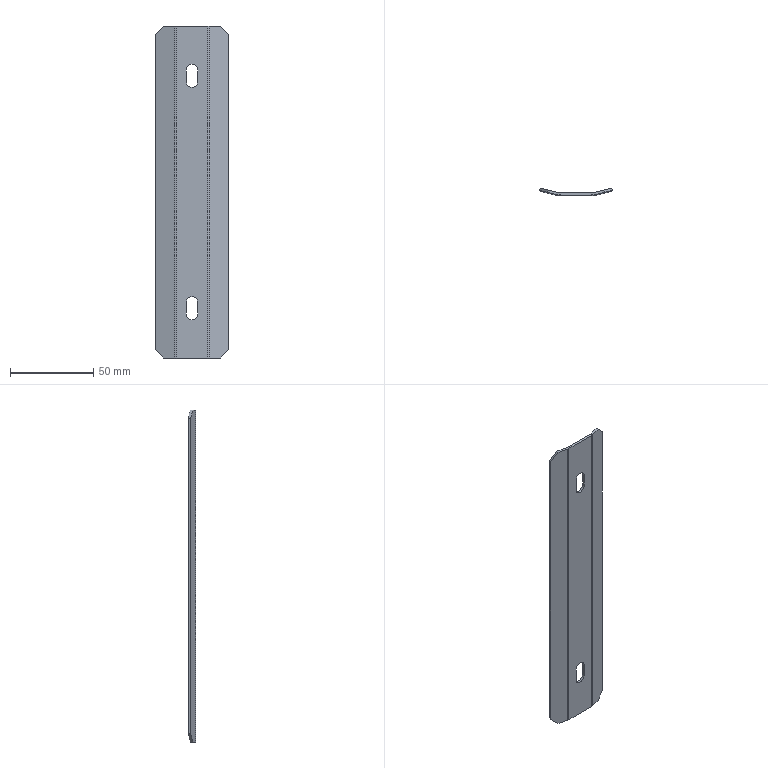Part | STEP file | SYL_0392D6J1SYL0380DJ1006_2_6-1 | 1 solid | 38 faces | box 44 x 4.447 x 200 mm | volume 12970 mm3 | plane 26 | cylinder 12 | commonest cylinder face diameters 7 x10 4 x2
STEP:
#1=CARTESIAN_POINT('',(-3.5,0.,-66.5));
#2=VERTEX_POINT('',#1);
#3=CARTESIAN_POINT('',(-3.5,1.5,-66.5));
#4=VERTEX_POINT('',#3);
#5=CARTESIAN_POINT('',(-3.5,1.5,-66.5));
#6=DIRECTION('',(0.,1.,0.));
#7=VECTOR('',#6,1000.);
#8=LINE('',#5,#7);
#9=EDGE_CURVE('',#2,#4,#8,.T.);
#10=ORIENTED_EDGE('',*,*,#9,.F.);
#11=CARTESIAN_POINT('',(-3.5,0.,-73.5));
#12=VERTEX_POINT('',#11);
#13=CARTESIAN_POINT('',(-3.5,0.,-100.));
#14=DIRECTION('',(0.,0.,-1.));
#15=VECTOR('',#14,1000.);
#16=LINE('',#13,#15);
#17=EDGE_CURVE('',#2,#12,#16,.T.);
#18=ORIENTED_EDGE('',*,*,#17,.T.);
#19=CARTESIAN_POINT('',(-3.5,1.5,-73.5));
#20=VERTEX_POINT('',#19);
#21=CARTESIAN_POINT('',(-3.5,1.5,-73.5));
#22=DIRECTION('',(0.,1.,0.));
#23=VECTOR('',#22,1000.);
#24=LINE('',#21,#23);
#25=EDGE_CURVE('',#12,#20,#24,.T.);
#26=ORIENTED_EDGE('',*,*,#25,.T.);
#27=CARTESIAN_POINT('',(-3.5,1.5,-66.5));
#28=DIRECTION('',(0.,0.,-1.));
#29=VECTOR('',#28,1000.);
#30=LINE('',#27,#29);
#31=EDGE_CURVE('',#4,#20,#30,.T.);
#32=ORIENTED_EDGE('',*,*,#31,.F.);
#33=EDGE_LOOP('',(#10,#18,#26,#32));
#34=FACE_OUTER_BOUND('',#33,.T.);
#35=CARTESIAN_POINT('',(-3.5,1.5,-66.5));
#36=DIRECTION('',(-1.,0.,0.));
#37=DIRECTION('',(0.,0.,-1.));
#38=AXIS2_PLACEMENT_3D('',#35,#36,#37);
#39=PLANE('',#38);
#40=ADVANCED_FACE('',(#34),#39,.F.);
#41=ORIENTED_EDGE('',*,*,#25,.F.);
#42=CARTESIAN_POINT('',(0.,0.,-77.));
#43=VERTEX_POINT('',#42);
#44=CARTESIAN_POINT('',(0.,0.,-73.5));
#45=DIRECTION('',(0.,-1.,0.));
#46=DIRECTION('',(0.,0.,-1.));
#47=AXIS2_PLACEMENT_3D('',#44,#45,#46);
#48=CIRCLE('',#47,3.5);
#49=EDGE_CURVE('',#12,#43,#48,.T.);
#50=ORIENTED_EDGE('',*,*,#49,.T.);
#51=CARTESIAN_POINT('',(0.,1.5,-77.));
#52=VERTEX_POINT('',#51);
#53=CARTESIAN_POINT('',(0.,1.5,-77.));
#54=DIRECTION('',(0.,1.,0.));
#55=VECTOR('',#54,1000.);
#56=LINE('',#53,#55);
#57=EDGE_CURVE('',#43,#52,#56,.T.);
#58=ORIENTED_EDGE('',*,*,#57,.T.);
#59=CARTESIAN_POINT('',(0.,1.5,-73.5));
#60=DIRECTION('',(0.,-1.,0.));
#61=DIRECTION('',(-1.,0.,0.));
#62=AXIS2_PLACEMENT_3D('',#59,#60,#61);
#63=CIRCLE('',#62,3.5);
#64=EDGE_CURVE('',#20,#52,#63,.T.);
#65=ORIENTED_EDGE('',*,*,#64,.F.);
#66=EDGE_LOOP('',(#41,#50,#58,#65));
#67=FACE_OUTER_BOUND('',#66,.T.);
#68=CARTESIAN_POINT('',(0.,1.5,-73.5));
#69=DIRECTION('',(0.,-1.,0.));
#70=DIRECTION('',(0.,0.,-1.));
#71=AXIS2_PLACEMENT_3D('',#68,#69,#70);
#72=CYLINDRICAL_SURFACE('',#71,3.5);
#73=ADVANCED_FACE('',(#67),#72,.F.);
#74=ORIENTED_EDGE('',*,*,#57,.F.);
#75=CARTESIAN_POINT('',(3.5,0.,-73.5));
#76=VERTEX_POINT('',#75);
#77=CARTESIAN_POINT('',(0.,0.,-73.5));
#78=DIRECTION('',(0.,-1.,0.));
#79=DIRECTION('',(0.,0.,-1.));
#80=AXIS2_PLACEMENT_3D('',#77,#78,#79);
#81=CIRCLE('',#80,3.5);
#82=EDGE_CURVE('',#43,#76,#81,.T.);
#83=ORIENTED_EDGE('',*,*,#82,.T.);
#84=CARTESIAN_POINT('',(3.5,1.5,-73.5));
#85=VERTEX_POINT('',#84);
#86=CARTESIAN_POINT('',(3.5,1.5,-73.5));
#87=DIRECTION('',(0.,1.,0.));
#88=VECTOR('',#87,1000.);
#89=LINE('',#86,#88);
#90=EDGE_CURVE('',#76,#85,#89,.T.);
#91=ORIENTED_EDGE('',*,*,#90,.T.);
#92=CARTESIAN_POINT('',(0.,1.5,-73.5));
#93=DIRECTION('',(0.,-1.,0.));
#94=DIRECTION('',(0.,0.,-1.));
#95=AXIS2_PLACEMENT_3D('',#92,#93,#94);
#96=CIRCLE('',#95,3.5);
#97=EDGE_CURVE('',#52,#85,#96,.T.);
#98=ORIENTED_EDGE('',*,*,#97,.F.);
#99=EDGE_LOOP('',(#74,#83,#91,#98));
#100=FACE_OUTER_BOUND('',#99,.T.);
#101=CARTESIAN_POINT('',(0.,1.5,-73.5));
#102=DIRECTION('',(0.,-1.,0.));
#103=DIRECTION('',(0.,0.,-1.));
#104=AXIS2_PLACEMENT_3D('',#101,#102,#103);
#105=CYLINDRICAL_SURFACE('',#104,3.5);
#106=ADVANCED_FACE('',(#100),#105,.F.);
#107=ORIENTED_EDGE('',*,*,#90,.F.);
#108=CARTESIAN_POINT('',(3.5,0.,-66.5));
#109=VERTEX_POINT('',#108);
#110=CARTESIAN_POINT('',(3.5,0.,-100.));
#111=DIRECTION('',(0.,0.,1.));
#112=VECTOR('',#111,1000.);
#113=LINE('',#110,#112);
#114=EDGE_CURVE('',#76,#109,#113,.T.);
#115=ORIENTED_EDGE('',*,*,#114,.T.);
#116=CARTESIAN_POINT('',(3.5,1.5,-66.5));
#117=VERTEX_POINT('',#116);
#118=CARTESIAN_POINT('',(3.5,1.5,-66.5));
#119=DIRECTION('',(0.,1.,0.));
#120=VECTOR('',#119,1000.);
#121=LINE('',#118,#120);
#122=EDGE_CURVE('',#109,#117,#121,.T.);
#123=ORIENTED_EDGE('',*,*,#122,.T.);
#124=CARTESIAN_POINT('',(3.5,1.5,-73.5));
#125=DIRECTION('',(0.,0.,1.));
#126=VECTOR('',#125,1000.);
#127=LINE('',#124,#126);
#128=EDGE_CURVE('',#85,#117,#127,.T.);
#129=ORIENTED_EDGE('',*,*,#128,.F.);
#130=EDGE_LOOP('',(#107,#115,#123,#129));
#131=FACE_OUTER_BOUND('',#130,.T.);
#132=CARTESIAN_POINT('',(3.5,1.5,-73.5));
#133=DIRECTION('',(1.,0.,0.));
#134=DIRECTION('',(0.,0.,1.));
#135=AXIS2_PLACEMENT_3D('',#132,#133,#134);
#136=PLANE('',#135);
#137=ADVANCED_FACE('',(#131),#136,.F.);
#138=ORIENTED_EDGE('',*,*,#122,.F.);
#139=CARTESIAN_POINT('',(0.,0.,-63.));
#140=VERTEX_POINT('',#139);
#141=CARTESIAN_POINT('',(0.,0.,-66.5));
#142=DIRECTION('',(0.,-1.,0.));
#143=DIRECTION('',(0.,0.,-1.));
#144=AXIS2_PLACEMENT_3D('',#141,#142,#143);
#145=CIRCLE('',#144,3.5);
#146=EDGE_CURVE('',#109,#140,#145,.T.);
#147=ORIENTED_EDGE('',*,*,#146,.T.);
#148=CARTESIAN_POINT('',(0.,1.5,-63.));
#149=VERTEX_POINT('',#148);
#150=CARTESIAN_POINT('',(0.,1.5,-63.));
#151=DIRECTION('',(0.,1.,0.));
#152=VECTOR('',#151,1000.);
#153=LINE('',#150,#152);
#154=EDGE_CURVE('',#140,#149,#153,.T.);
#155=ORIENTED_EDGE('',*,*,#154,.T.);
#156=CARTESIAN_POINT('',(0.,1.5,-66.5));
#157=DIRECTION('',(0.,-1.,0.));
#158=DIRECTION('',(1.,0.,0.));
#159=AXIS2_PLACEMENT_3D('',#156,#157,#158);
#160=CIRCLE('',#159,3.5);
#161=EDGE_CURVE('',#117,#149,#160,.T.);
#162=ORIENTED_EDGE('',*,*,#161,.F.);
#163=EDGE_LOOP('',(#138,#147,#155,#162));
#164=FACE_OUTER_BOUND('',#163,.T.);
#165=CARTESIAN_POINT('',(0.,1.5,-66.5));
#166=DIRECTION('',(0.,-1.,0.));
#167=DIRECTION('',(0.,0.,-1.));
#168=AXIS2_PLACEMENT_3D('',#165,#166,#167);
#169=CYLINDRICAL_SURFACE('',#168,3.5);
#170=ADVANCED_FACE('',(#164),#169,.F.);
#171=CARTESIAN_POINT('',(-3.5,0.,73.5));
#172=VERTEX_POINT('',#171);
#173=CARTESIAN_POINT('',(-3.5,1.5,73.5));
#174=VERTEX_POINT('',#173);
#175=CARTESIAN_POINT('',(-3.5,1.5,73.5));
#176=DIRECTION('',(0.,1.,0.));
#177=VECTOR('',#176,1000.);
#178=LINE('',#175,#177);
#179=EDGE_CURVE('',#172,#174,#178,.T.);
#180=ORIENTED_EDGE('',*,*,#179,.F.);
#181=CARTESIAN_POINT('',(-3.5,0.,66.5));
#182=VERTEX_POINT('',#181);
#183=CARTESIAN_POINT('',(-3.5,0.,-100.));
#184=DIRECTION('',(0.,0.,-1.));
#185=VECTOR('',#184,1000.);
#186=LINE('',#183,#185);
#187=EDGE_CURVE('',#172,#182,#186,.T.);
#188=ORIENTED_EDGE('',*,*,#187,.T.);
#189=CARTESIAN_POINT('',(-3.5,1.5,66.5));
#190=VERTEX_POINT('',#189);
#191=CARTESIAN_POINT('',(-3.5,1.5,66.5));
#192=DIRECTION('',(0.,1.,0.));
#193=VECTOR('',#192,1000.);
#194=LINE('',#191,#193);
#195=EDGE_CURVE('',#182,#190,#194,.T.);
#196=ORIENTED_EDGE('',*,*,#195,.T.);
#197=CARTESIAN_POINT('',(-3.5,1.5,73.5));
#198=DIRECTION('',(0.,0.,-1.));
#199=VECTOR('',#198,1000.);
#200=LINE('',#197,#199);
#201=EDGE_CURVE('',#174,#190,#200,.T.);
#202=ORIENTED_EDGE('',*,*,#201,.F.);
#203=EDGE_LOOP('',(#180,#188,#196,#202));
#204=FACE_OUTER_BOUND('',#203,.T.);
#205=CARTESIAN_POINT('',(-3.5,1.5,73.5));
#206=DIRECTION('',(-1.,0.,0.));
#207=DIRECTION('',(0.,0.,-1.));
#208=AXIS2_PLACEMENT_3D('',#205,#206,#207);
#209=PLANE('',#208);
#210=ADVANCED_FACE('',(#204),#209,.F.);
#211=ORIENTED_EDGE('',*,*,#195,.F.);
#212=CARTESIAN_POINT('',(0.,0.,63.));
#213=VERTEX_POINT('',#212);
#214=CARTESIAN_POINT('',(0.,0.,66.5));
#215=DIRECTION('',(0.,-1.,0.));
#216=DIRECTION('',(0.,0.,-1.));
#217=AXIS2_PLACEMENT_3D('',#214,#215,#216);
#218=CIRCLE('',#217,3.5);
#219=EDGE_CURVE('',#182,#213,#218,.T.);
#220=ORIENTED_EDGE('',*,*,#219,.T.);
#221=CARTESIAN_POINT('',(0.,1.5,63.));
#222=VERTEX_POINT('',#221);
#223=CARTESIAN_POINT('',(0.,1.5,63.));
#224=DIRECTION('',(0.,1.,0.));
#225=VECTOR('',#224,1000.);
#226=LINE('',#223,#225);
#227=EDGE_CURVE('',#213,#222,#226,.T.);
#228=ORIENTED_EDGE('',*,*,#227,.T.);
#229=CARTESIAN_POINT('',(0.,1.5,66.5));
#230=DIRECTION('',(0.,-1.,0.));
#231=DIRECTION('',(-1.,0.,0.));
#232=AXIS2_PLACEMENT_3D('',#229,#230,#231);
#233=CIRCLE('',#232,3.5);
#234=EDGE_CURVE('',#190,#222,#233,.T.);
#235=ORIENTED_EDGE('',*,*,#234,.F.);
#236=EDGE_LOOP('',(#211,#220,#228,#235));
#237=FACE_OUTER_BOUND('',#236,.T.);
#238=CARTESIAN_POINT('',(0.,1.5,66.5));
#239=DIRECTION('',(0.,-1.,0.));
#240=DIRECTION('',(0.,0.,-1.));
#241=AXIS2_PLACEMENT_3D('',#238,#239,#240);
#242=CYLINDRICAL_SURFACE('',#241,3.5);
#243=ADVANCED_FACE('',(#237),#242,.F.);
#244=ORIENTED_EDGE('',*,*,#227,.F.);
#245=CARTESIAN_POINT('',(3.5,0.,66.5));
#246=VERTEX_POINT('',#245);
#247=CARTESIAN_POINT('',(0.,0.,66.5));
#248=DIRECTION('',(0.,-1.,0.));
#249=DIRECTION('',(0.,0.,-1.));
#250=AXIS2_PLACEMENT_3D('',#247,#248,#249);
#251=CIRCLE('',#250,3.5);
#252=EDGE_CURVE('',#213,#246,#251,.T.);
#253=ORIENTED_EDGE('',*,*,#252,.T.);
#254=CARTESIAN_POINT('',(3.5,1.5,66.5));
#255=VERTEX_POINT('',#254);
#256=CARTESIAN_POINT('',(3.5,1.5,66.5));
#257=DIRECTION('',(0.,1.,0.));
#258=VECTOR('',#257,1000.);
#259=LINE('',#256,#258);
#260=EDGE_CURVE('',#246,#255,#259,.T.);
#261=ORIENTED_EDGE('',*,*,#260,.T.);
#262=CARTESIAN_POINT('',(0.,1.5,66.5));
#263=DIRECTION('',(0.,-1.,0.));
#264=DIRECTION('',(0.,0.,-1.));
#265=AXIS2_PLACEMENT_3D('',#262,#263,#264);
#266=CIRCLE('',#265,3.5);
#267=EDGE_CURVE('',#222,#255,#266,.T.);
#268=ORIENTED_EDGE('',*,*,#267,.F.);
#269=EDGE_LOOP('',(#244,#253,#261,#268));
#270=FACE_OUTER_BOUND('',#269,.T.);
#271=CARTESIAN_POINT('',(0.,1.5,66.5));
#272=DIRECTION('',(0.,-1.,0.));
#273=DIRECTION('',(0.,0.,-1.));
#274=AXIS2_PLACEMENT_3D('',#271,#272,#273);
#275=CYLINDRICAL_SURFACE('',#274,3.5);
#276=ADVANCED_FACE('',(#270),#275,.F.);
#277=ORIENTED_EDGE('',*,*,#260,.F.);
#278=CARTESIAN_POINT('',(3.5,0.,73.5));
#279=VERTEX_POINT('',#278);
#280=CARTESIAN_POINT('',(3.5,0.,-100.));
#281=DIRECTION('',(0.,0.,1.));
#282=VECTOR('',#281,1000.);
#283=LINE('',#280,#282);
#284=EDGE_CURVE('',#246,#279,#283,.T.);
#285=ORIENTED_EDGE('',*,*,#284,.T.);
#286=CARTESIAN_POINT('',(3.5,1.5,73.5));
#287=VERTEX_POINT('',#286);
#288=CARTESIAN_POINT('',(3.5,1.5,73.5));
#289=DIRECTION('',(0.,1.,0.));
#290=VECTOR('',#289,1000.);
#291=LINE('',#288,#290);
#292=EDGE_CURVE('',#279,#287,#291,.T.);
#293=ORIENTED_EDGE('',*,*,#292,.T.);
#294=CARTESIAN_POINT('',(3.5,1.5,66.5));
#295=DIRECTION('',(0.,0.,1.));
#296=VECTOR('',#295,1000.);
#297=LINE('',#294,#296);
#298=EDGE_CURVE('',#255,#287,#297,.T.);
#299=ORIENTED_EDGE('',*,*,#298,.F.);
#300=EDGE_LOOP('',(#277,#285,#293,#299));
#301=FACE_OUTER_BOUND('',#300,.T.);
#302=CARTESIAN_POINT('',(3.5,1.5,66.5));
#303=DIRECTION('',(1.,0.,0.));
#304=DIRECTION('',(0.,0.,1.));
#305=AXIS2_PLACEMENT_3D('',#302,#303,#304);
#306=PLANE('',#305);
#307=ADVANCED_FACE('',(#301),#306,.F.);
#308=ORIENTED_EDGE('',*,*,#292,.F.);
#309=CARTESIAN_POINT('',(0.,0.,77.));
#310=VERTEX_POINT('',#309);
#311=CARTESIAN_POINT('',(0.,0.,73.5));
#312=DIRECTION('',(0.,-1.,0.));
#313=DIRECTION('',(0.,0.,-1.));
#314=AXIS2_PLACEMENT_3D('',#311,#312,#313);
#315=CIRCLE('',#314,3.5);
#316=EDGE_CURVE('',#279,#310,#315,.T.);
#317=ORIENTED_EDGE('',*,*,#316,.T.);
#318=CARTESIAN_POINT('',(0.,1.5,77.));
#319=VERTEX_POINT('',#318);
#320=CARTESIAN_POINT('',(0.,1.5,77.));
#321=DIRECTION('',(0.,1.,0.));
#322=VECTOR('',#321,1000.);
#323=LINE('',#320,#322);
#324=EDGE_CURVE('',#310,#319,#323,.T.);
#325=ORIENTED_EDGE('',*,*,#324,.T.);
#326=CARTESIAN_POINT('',(0.,1.5,73.5));
#327=DIRECTION('',(0.,-1.,0.));
#328=DIRECTION('',(1.,0.,0.));
#329=AXIS2_PLACEMENT_3D('',#326,#327,#328);
#330=CIRCLE('',#329,3.5);
#331=EDGE_CURVE('',#287,#319,#330,.T.);
#332=ORIENTED_EDGE('',*,*,#331,.F.);
#333=EDGE_LOOP('',(#308,#317,#325,#332));
#334=FACE_OUTER_BOUND('',#333,.T.);
#335=CARTESIAN_POINT('',(0.,1.5,73.5));
#336=DIRECTION('',(0.,-1.,0.));
#337=DIRECTION('',(0.,0.,-1.));
#338=AXIS2_PLACEMENT_3D('',#335,#336,#337);
#339=CYLINDRICAL_SURFACE('',#338,3.5);
#340=ADVANCED_FACE('',(#334),#339,.F.);
#341=CARTESIAN_POINT('',(-17.149,1.782,-100.));
#342=VERTEX_POINT('',#341);
#343=CARTESIAN_POINT('',(-16.786,3.238,-100.));
#344=VERTEX_POINT('',#343);
#345=CARTESIAN_POINT('',(-16.786,3.238,-100.));
#346=DIRECTION('',(0.2419,0.9703,0.));
#347=VECTOR('',#346,1000.);
#348=LINE('',#345,#347);
#349=EDGE_CURVE('',#342,#344,#348,.T.);
#350=ORIENTED_EDGE('',*,*,#349,.F.);
#351=CARTESIAN_POINT('',(-22.,2.992,-95.));
#352=VERTEX_POINT('',#351);
#353=CARTESIAN_POINT('',(-17.149,1.782,-100.));
#354=DIRECTION('',(-0.6861,0.1711,0.7071));
#355=VECTOR('',#354,1000.);
#356=LINE('',#353,#355);
#357=EDGE_CURVE('',#342,#352,#356,.T.);
#358=ORIENTED_EDGE('',*,*,#357,.T.);
#359=CARTESIAN_POINT('',(-21.637,4.447,-95.));
#360=VERTEX_POINT('',#359);
#361=CARTESIAN_POINT('',(-21.637,4.447,-95.));
#362=DIRECTION('',(0.2419,0.9703,0.));
#363=VECTOR('',#362,1000.);
#364=LINE('',#361,#363);
#365=EDGE_CURVE('',#352,#360,#364,.T.);
#366=ORIENTED_EDGE('',*,*,#365,.T.);
#367=CARTESIAN_POINT('',(-16.786,3.238,-100.));
#368=DIRECTION('',(-0.6861,0.1711,0.7071));
#369=VECTOR('',#368,1000.);
#370=LINE('',#367,#369);
#371=EDGE_CURVE('',#344,#360,#370,.T.);
#372=ORIENTED_EDGE('',*,*,#371,.F.);
#373=EDGE_LOOP('',(#350,#358,#366,#372));
#374=FACE_OUTER_BOUND('',#373,.T.);
#375=CARTESIAN_POINT('',(-16.786,3.238,-100.));
#376=DIRECTION('',(0.6861,-0.1711,0.7071));
#377=DIRECTION('',(-0.6861,0.1711,0.7071));
#378=AXIS2_PLACEMENT_3D('',#375,#376,#377);
#379=PLANE('',#378);
#380=ADVANCED_FACE('',(#374),#379,.F.);
#381=ORIENTED_EDGE('',*,*,#365,.F.);
#382=CARTESIAN_POINT('',(-22.,2.992,95.));
#383=VERTEX_POINT('',#382);
#384=CARTESIAN_POINT('',(-22.,2.992,-100.));
#385=DIRECTION('',(0.,0.,1.));
#386=VECTOR('',#385,1000.);
#387=LINE('',#384,#386);
#388=EDGE_CURVE('',#352,#383,#387,.T.);
#389=ORIENTED_EDGE('',*,*,#388,.T.);
#390=CARTESIAN_POINT('',(-21.637,4.447,95.));
#391=VERTEX_POINT('',#390);
#392=CARTESIAN_POINT('',(-21.637,4.447,95.));
#393=DIRECTION('',(0.2419,0.9703,0.));
#394=VECTOR('',#393,1000.);
#395=LINE('',#392,#394);
#396=EDGE_CURVE('',#383,#391,#395,.T.);
#397=ORIENTED_EDGE('',*,*,#396,.T.);
#398=CARTESIAN_POINT('',(-21.637,4.447,-95.));
#399=DIRECTION('',(0.,0.,1.));
#400=VECTOR('',#399,1000.);
#401=LINE('',#398,#400);
#402=EDGE_CURVE('',#360,#391,#401,.T.);
#403=ORIENTED_EDGE('',*,*,#402,.F.);
#404=EDGE_LOOP('',(#381,#389,#397,#403));
#405=FACE_OUTER_BOUND('',#404,.T.);
#406=CARTESIAN_POINT('',(-21.637,4.447,-95.));
#407=DIRECTION('',(0.9703,-0.2419,0.));
#408=DIRECTION('',(0.,0.,1.));
#409=AXIS2_PLACEMENT_3D('',#406,#407,#408);
#410=PLANE('',#409);
#411=ADVANCED_FACE('',(#405),#410,.F.);
#412=ORIENTED_EDGE('',*,*,#396,.F.);
#413=CARTESIAN_POINT('',(-17.149,1.782,100.));
#414=VERTEX_POINT('',#413);
#415=CARTESIAN_POINT('',(-22.,2.992,95.));
#416=DIRECTION('',(0.6861,-0.1711,0.7071));
#417=VECTOR('',#416,1000.);
#418=LINE('',#415,#417);
#419=EDGE_CURVE('',#383,#414,#418,.T.);
#420=ORIENTED_EDGE('',*,*,#419,.T.);
#421=CARTESIAN_POINT('',(-16.786,3.238,100.));
#422=VERTEX_POINT('',#421);
#423=CARTESIAN_POINT('',(-16.786,3.238,100.));
#424=DIRECTION('',(0.2419,0.9703,0.));
#425=VECTOR('',#424,1000.);
#426=LINE('',#423,#425);
#427=EDGE_CURVE('',#414,#422,#426,.T.);
#428=ORIENTED_EDGE('',*,*,#427,.T.);
#429=CARTESIAN_POINT('',(-21.637,4.447,95.));
#430=DIRECTION('',(0.6861,-0.1711,0.7071));
#431=VECTOR('',#430,1000.);
#432=LINE('',#429,#431);
#433=EDGE_CURVE('',#391,#422,#432,.T.);
#434=ORIENTED_EDGE('',*,*,#433,.F.);
#435=EDGE_LOOP('',(#412,#420,#428,#434));
#436=FACE_OUTER_BOUND('',#435,.T.);
#437=CARTESIAN_POINT('',(-21.637,4.447,95.));
#438=DIRECTION('',(0.6861,-0.1711,-0.7071));
#439=DIRECTION('',(0.6861,-0.1711,0.7071));
#440=AXIS2_PLACEMENT_3D('',#437,#438,#439);
#441=PLANE('',#440);
#442=ADVANCED_FACE('',(#436),#441,.F.);
#443=ORIENTED_EDGE('',*,*,#427,.F.);
#444=CARTESIAN_POINT('',(-10.417,0.104,100.));
#445=VERTEX_POINT('',#444);
#446=CARTESIAN_POINT('',(-22.,2.992,100.));
#447=DIRECTION('',(-0.9703,0.2419,0.));
#448=VECTOR('',#447,1000.);
#449=LINE('',#446,#448);
#450=EDGE_CURVE('',#445,#414,#449,.T.);
#451=ORIENTED_EDGE('',*,*,#450,.F.);
#452=CARTESIAN_POINT('',(-10.054,1.559,100.));
#453=VERTEX_POINT('',#452);
#454=CARTESIAN_POINT('',(-10.054,1.559,100.));
#455=DIRECTION('',(0.2419,0.9703,0.));
#456=VECTOR('',#455,1000.);
#457=LINE('',#454,#456);
#458=EDGE_CURVE('',#445,#453,#457,.T.);
#459=ORIENTED_EDGE('',*,*,#458,.T.);
#460=CARTESIAN_POINT('',(-10.054,1.559,100.));
#461=DIRECTION('',(-0.9703,0.2419,0.));
#462=VECTOR('',#461,1000.);
#463=LINE('',#460,#462);
#464=EDGE_CURVE('',#453,#422,#463,.T.);
#465=ORIENTED_EDGE('',*,*,#464,.T.);
#466=EDGE_LOOP('',(#443,#451,#459,#465));
#467=FACE_OUTER_BOUND('',#466,.T.);
#468=CARTESIAN_POINT('',(-10.054,1.559,100.));
#469=DIRECTION('',(0.,0.,1.));
#470=DIRECTION('',(-0.9703,0.2419,0.));
#471=AXIS2_PLACEMENT_3D('',#468,#469,#470);
#472=PLANE('',#471);
#473=ADVANCED_FACE('',(#467),#472,.T.);
#474=ORIENTED_EDGE('',*,*,#458,.F.);
#475=CARTESIAN_POINT('',(-9.57,0.,100.));
#476=VERTEX_POINT('',#475);
#477=CARTESIAN_POINT('',(-9.57,3.5,100.));
#478=DIRECTION('',(0.,0.,-1.));
#479=DIRECTION('',(1.,0.,0.));
#480=AXIS2_PLACEMENT_3D('',#477,#478,#479);
#481=CIRCLE('',#480,3.5);
#482=EDGE_CURVE('',#476,#445,#481,.T.);
#483=ORIENTED_EDGE('',*,*,#482,.F.);
#484=CARTESIAN_POINT('',(-9.57,1.5,100.));
#485=VERTEX_POINT('',#484);
#486=CARTESIAN_POINT('',(-9.57,1.5,100.));
#487=DIRECTION('',(0.,1.,0.));
#488=VECTOR('',#487,1000.);
#489=LINE('',#486,#488);
#490=EDGE_CURVE('',#476,#485,#489,.T.);
#491=ORIENTED_EDGE('',*,*,#490,.T.);
#492=CARTESIAN_POINT('',(-9.57,3.5,100.));
#493=DIRECTION('',(0.,0.,-1.));
#494=DIRECTION('',(0.,-1.,0.));
#495=AXIS2_PLACEMENT_3D('',#492,#493,#494);
#496=CIRCLE('',#495,2.);
#497=EDGE_CURVE('',#485,#453,#496,.T.);
#498=ORIENTED_EDGE('',*,*,#497,.T.);
#499=EDGE_LOOP('',(#474,#483,#491,#498));
#500=FACE_OUTER_BOUND('',#499,.T.);
#501=CARTESIAN_POINT('',(-9.57,3.5,100.));
#502=DIRECTION('',(0.,0.,1.));
#503=DIRECTION('',(1.,0.,0.));
#504=AXIS2_PLACEMENT_3D('',#501,#502,#503);
#505=PLANE('',#504);
#506=ADVANCED_FACE('',(#500),#505,.T.);
#507=ORIENTED_EDGE('',*,*,#490,.F.);
#508=CARTESIAN_POINT('',(9.57,0.,100.));
#509=VERTEX_POINT('',#508);
#510=CARTESIAN_POINT('',(-9.57,0.,100.));
#511=DIRECTION('',(1.,0.,0.));
#512=VECTOR('',#511,1000.);
#513=LINE('',#510,#512);
#514=EDGE_CURVE('',#476,#509,#513,.T.);
#515=ORIENTED_EDGE('',*,*,#514,.T.);
#516=CARTESIAN_POINT('',(9.57,1.5,100.));
#517=VERTEX_POINT('',#516);
#518=CARTESIAN_POINT('',(9.57,0.,100.));
#519=CARTESIAN_POINT('',(9.57,0.5,100.));
#520=CARTESIAN_POINT('',(9.57,1.,100.));
#521=CARTESIAN_POINT('',(9.57,1.5,100.));
#522=B_SPLINE_CURVE_WITH_KNOTS('',3,(#518,#519,#520,#521),.UNSPECIFIED.,.F.,.F.,(4,4),(0.,1.),.UNSPECIFIED.);
#523=EDGE_CURVE('',#509,#517,#522,.T.);
#524=ORIENTED_EDGE('',*,*,#523,.T.);
#525=CARTESIAN_POINT('',(-9.57,1.5,100.));
#526=DIRECTION('',(1.,0.,0.));
#527=VECTOR('',#526,1000.);
#528=LINE('',#525,#527);
#529=EDGE_CURVE('',#485,#517,#528,.T.);
#530=ORIENTED_EDGE('',*,*,#529,.F.);
#531=EDGE_LOOP('',(#507,#515,#524,#530));
#532=FACE_OUTER_BOUND('',#531,.T.);
#533=CARTESIAN_POINT('',(-9.57,1.5,100.));
#534=DIRECTION('',(0.,0.,-1.));
#535=DIRECTION('',(1.,0.,0.));
#536=AXIS2_PLACEMENT_3D('',#533,#534,#535);
#537=PLANE('',#536);
#538=ADVANCED_FACE('',(#532),#537,.F.);
#539=ORIENTED_EDGE('',*,*,#523,.F.);
#540=CARTESIAN_POINT('',(10.421,0.1051,100.));
#541=VERTEX_POINT('',#540);
#542=CARTESIAN_POINT('',(10.421,0.1051,100.));
#543=CARTESIAN_POINT('',(10.143,0.03537,100.));
#544=CARTESIAN_POINT('',(9.857,0.,100.));
#545=CARTESIAN_POINT('',(9.57,0.,100.));
#546=B_SPLINE_CURVE_WITH_KNOTS('',3,(#542,#543,#544,#545),.UNSPECIFIED.,.F.,.F.,(4,4),(0.,1.),.UNSPECIFIED.);
#547=EDGE_CURVE('',#541,#509,#546,.T.);
#548=ORIENTED_EDGE('',*,*,#547,.F.);
#549=CARTESIAN_POINT('',(10.057,1.56,100.));
#550=VERTEX_POINT('',#549);
#551=CARTESIAN_POINT('',(10.421,0.1051,100.));
#552=CARTESIAN_POINT('',(10.3,0.59,100.));
#553=CARTESIAN_POINT('',(10.178,1.075,100.));
#554=CARTESIAN_POINT('',(10.057,1.56,100.));
#555=B_SPLINE_CURVE_WITH_KNOTS('',3,(#551,#552,#553,#554),.UNSPECIFIED.,.F.,.F.,(4,4),(0.,1.),.UNSPECIFIED.);
#556=EDGE_CURVE('',#541,#550,#555,.T.);
#557=ORIENTED_EDGE('',*,*,#556,.T.);
#558=CARTESIAN_POINT('',(10.057,1.56,100.));
#559=CARTESIAN_POINT('',(9.897,1.52,100.));
#560=CARTESIAN_POINT('',(9.735,1.5,100.));
#561=CARTESIAN_POINT('',(9.57,1.5,100.));
#562=B_SPLINE_CURVE_WITH_KNOTS('',3,(#558,#559,#560,#561),.UNSPECIFIED.,.F.,.F.,(4,4),(0.,1.),.UNSPECIFIED.);
#563=EDGE_CURVE('',#550,#517,#562,.T.);
#564=ORIENTED_EDGE('',*,*,#563,.T.);
#565=EDGE_LOOP('',(#539,#548,#557,#564));
#566=FACE_OUTER_BOUND('',#565,.T.);
#567=CARTESIAN_POINT('',(9.57,3.5,100.));
#568=DIRECTION('',(0.,0.,-1.));
#569=DIRECTION('',(-1.,0.,0.));
#570=AXIS2_PLACEMENT_3D('',#567,#568,#569);
#571=PLANE('',#570);
#572=ADVANCED_FACE('',(#566),#571,.F.);
#573=ORIENTED_EDGE('',*,*,#556,.F.);
#574=CARTESIAN_POINT('',(17.149,1.782,100.));
#575=VERTEX_POINT('',#574);
#576=CARTESIAN_POINT('',(10.417,0.104,100.));
#577=DIRECTION('',(-0.9703,-0.2419,0.));
#578=VECTOR('',#577,1000.);
#579=LINE('',#576,#578);
#580=EDGE_CURVE('',#575,#541,#579,.T.);
#581=ORIENTED_EDGE('',*,*,#580,.F.);
#582=CARTESIAN_POINT('',(16.786,3.238,100.));
#583=VERTEX_POINT('',#582);
#584=CARTESIAN_POINT('',(16.786,3.238,100.));
#585=DIRECTION('',(-0.2419,0.9703,0.));
#586=VECTOR('',#585,1000.);
#587=LINE('',#584,#586);
#588=EDGE_CURVE('',#575,#583,#587,.T.);
#589=ORIENTED_EDGE('',*,*,#588,.T.);
#590=CARTESIAN_POINT('',(16.786,3.238,100.));
#591=DIRECTION('',(-0.9703,-0.2419,0.));
#592=VECTOR('',#591,1000.);
#593=LINE('',#590,#592);
#594=EDGE_CURVE('',#583,#550,#593,.T.);
#595=ORIENTED_EDGE('',*,*,#594,.T.);
#596=EDGE_LOOP('',(#573,#581,#589,#595));
#597=FACE_OUTER_BOUND('',#596,.T.);
#598=CARTESIAN_POINT('',(16.786,3.238,100.));
#599=DIRECTION('',(0.,0.,1.));
#600=DIRECTION('',(-0.9703,-0.2419,0.));
#601=AXIS2_PLACEMENT_3D('',#598,#599,#600);
#602=PLANE('',#601);
#603=ADVANCED_FACE('',(#597),#602,.T.);
#604=ORIENTED_EDGE('',*,*,#588,.F.);
#605=CARTESIAN_POINT('',(22.,2.992,95.));
#606=VERTEX_POINT('',#605);
#607=CARTESIAN_POINT('',(17.149,1.782,100.));
#608=DIRECTION('',(0.6861,0.1711,-0.7071));
#609=VECTOR('',#608,1000.);
#610=LINE('',#607,#609);
#611=EDGE_CURVE('',#575,#606,#610,.T.);
#612=ORIENTED_EDGE('',*,*,#611,.T.);
#613=CARTESIAN_POINT('',(21.637,4.447,95.));
#614=VERTEX_POINT('',#613);
#615=CARTESIAN_POINT('',(21.637,4.447,95.));
#616=DIRECTION('',(-0.2419,0.9703,0.));
#617=VECTOR('',#616,1000.);
#618=LINE('',#615,#617);
#619=EDGE_CURVE('',#606,#614,#618,.T.);
#620=ORIENTED_EDGE('',*,*,#619,.T.);
#621=CARTESIAN_POINT('',(16.786,3.238,100.));
#622=DIRECTION('',(0.6861,0.1711,-0.7071));
#623=VECTOR('',#622,1000.);
#624=LINE('',#621,#623);
#625=EDGE_CURVE('',#583,#614,#624,.T.);
#626=ORIENTED_EDGE('',*,*,#625,.F.);
#627=EDGE_LOOP('',(#604,#612,#620,#626));
#628=FACE_OUTER_BOUND('',#627,.T.);
#629=CARTESIAN_POINT('',(16.786,3.238,100.));
#630=DIRECTION('',(-0.6861,-0.1711,-0.7071));
#631=DIRECTION('',(0.6861,0.1711,-0.7071));
#632=AXIS2_PLACEMENT_3D('',#629,#630,#631);
#633=PLANE('',#632);
#634=ADVANCED_FACE('',(#628),#633,.F.);
#635=ORIENTED_EDGE('',*,*,#619,.F.);
#636=CARTESIAN_POINT('',(22.,2.992,-95.));
#637=VERTEX_POINT('',#636);
#638=CARTESIAN_POINT('',(22.,2.992,-100.));
#639=DIRECTION('',(0.,0.,-1.));
#640=VECTOR('',#639,1000.);
#641=LINE('',#638,#640);
#642=EDGE_CURVE('',#606,#637,#641,.T.);
#643=ORIENTED_EDGE('',*,*,#642,.T.);
#644=CARTESIAN_POINT('',(21.637,4.447,-95.));
#645=VERTEX_POINT('',#644);
#646=CARTESIAN_POINT('',(21.637,4.447,-95.));
#647=DIRECTION('',(-0.2419,0.9703,0.));
#648=VECTOR('',#647,1000.);
#649=LINE('',#646,#648);
#650=EDGE_CURVE('',#637,#645,#649,.T.);
#651=ORIENTED_EDGE('',*,*,#650,.T.);
#652=CARTESIAN_POINT('',(21.637,4.447,95.));
#653=DIRECTION('',(0.,0.,-1.));
#654=VECTOR('',#653,1000.);
#655=LINE('',#652,#654);
#656=EDGE_CURVE('',#614,#645,#655,.T.);
#657=ORIENTED_EDGE('',*,*,#656,.F.);
#658=EDGE_LOOP('',(#635,#643,#651,#657));
#659=FACE_OUTER_BOUND('',#658,.T.);
#660=CARTESIAN_POINT('',(21.637,4.447,95.));
#661=DIRECTION('',(-0.9703,-0.2419,0.));
#662=DIRECTION('',(0.,0.,-1.));
#663=AXIS2_PLACEMENT_3D('',#660,#661,#662);
#664=PLANE('',#663);
#665=ADVANCED_FACE('',(#659),#664,.F.);
#666=ORIENTED_EDGE('',*,*,#650,.F.);
#667=CARTESIAN_POINT('',(17.149,1.782,-100.));
#668=VERTEX_POINT('',#667);
#669=CARTESIAN_POINT('',(22.,2.992,-95.));
#670=DIRECTION('',(-0.6861,-0.1711,-0.7071));
#671=VECTOR('',#670,1000.);
#672=LINE('',#669,#671);
#673=EDGE_CURVE('',#637,#668,#672,.T.);
#674=ORIENTED_EDGE('',*,*,#673,.T.);
#675=CARTESIAN_POINT('',(16.786,3.238,-100.));
#676=VERTEX_POINT('',#675);
#677=CARTESIAN_POINT('',(16.786,3.238,-100.));
#678=DIRECTION('',(-0.2419,0.9703,0.));
#679=VECTOR('',#678,1000.);
#680=LINE('',#677,#679);
#681=EDGE_CURVE('',#668,#676,#680,.T.);
#682=ORIENTED_EDGE('',*,*,#681,.T.);
#683=CARTESIAN_POINT('',(21.637,4.447,-95.));
#684=DIRECTION('',(-0.6861,-0.1711,-0.7071));
#685=VECTOR('',#684,1000.);
#686=LINE('',#683,#685);
#687=EDGE_CURVE('',#645,#676,#686,.T.);
#688=ORIENTED_EDGE('',*,*,#687,.F.);
#689=EDGE_LOOP('',(#666,#674,#682,#688));
#690=FACE_OUTER_BOUND('',#689,.T.);
#691=CARTESIAN_POINT('',(21.637,4.447,-95.));
#692=DIRECTION('',(-0.6861,-0.1711,0.7071));
#693=DIRECTION('',(-0.6861,-0.1711,-0.7071));
#694=AXIS2_PLACEMENT_3D('',#691,#692,#693);
#695=PLANE('',#694);
#696=ADVANCED_FACE('',(#690),#695,.F.);
#697=ORIENTED_EDGE('',*,*,#681,.F.);
#698=CARTESIAN_POINT('',(10.421,0.1051,-100.));
#699=VERTEX_POINT('',#698);
#700=CARTESIAN_POINT('',(10.417,0.104,-100.));
#701=DIRECTION('',(0.9703,0.2419,0.));
#702=VECTOR('',#701,1000.);
#703=LINE('',#700,#702);
#704=EDGE_CURVE('',#699,#668,#703,.T.);
#705=ORIENTED_EDGE('',*,*,#704,.F.);
#706=CARTESIAN_POINT('',(10.057,1.56,-100.));
#707=VERTEX_POINT('',#706);
#708=CARTESIAN_POINT('',(10.421,0.1051,-100.));
#709=CARTESIAN_POINT('',(10.3,0.59,-100.));
#710=CARTESIAN_POINT('',(10.178,1.075,-100.));
#711=CARTESIAN_POINT('',(10.057,1.56,-100.));
#712=B_SPLINE_CURVE_WITH_KNOTS('',3,(#708,#709,#710,#711),.UNSPECIFIED.,.F.,.F.,(4,4),(0.,1.),.UNSPECIFIED.);
#713=EDGE_CURVE('',#699,#707,#712,.T.);
#714=ORIENTED_EDGE('',*,*,#713,.T.);
#715=CARTESIAN_POINT('',(10.057,1.56,-100.));
#716=DIRECTION('',(0.9703,0.2419,0.));
#717=VECTOR('',#716,1000.);
#718=LINE('',#715,#717);
#719=EDGE_CURVE('',#707,#676,#718,.T.);
#720=ORIENTED_EDGE('',*,*,#719,.T.);
#721=EDGE_LOOP('',(#697,#705,#714,#720));
#722=FACE_OUTER_BOUND('',#721,.T.);
#723=CARTESIAN_POINT('',(10.057,1.56,-100.));
#724=DIRECTION('',(0.,0.,-1.));
#725=DIRECTION('',(0.9703,0.2419,0.));
#726=AXIS2_PLACEMENT_3D('',#723,#724,#725);
#727=PLANE('',#726);
#728=ADVANCED_FACE('',(#722),#727,.T.);
#729=ORIENTED_EDGE('',*,*,#713,.F.);
#730=CARTESIAN_POINT('',(9.57,0.,-100.));
#731=VERTEX_POINT('',#730);
#732=CARTESIAN_POINT('',(9.57,0.,-100.));
#733=CARTESIAN_POINT('',(9.857,0.,-100.));
#734=CARTESIAN_POINT('',(10.143,0.03537,-100.));
#735=CARTESIAN_POINT('',(10.421,0.1051,-100.));
#736=B_SPLINE_CURVE_WITH_KNOTS('',3,(#732,#733,#734,#735),.UNSPECIFIED.,.F.,.F.,(4,4),(0.,1.),.UNSPECIFIED.);
#737=EDGE_CURVE('',#731,#699,#736,.T.);
#738=ORIENTED_EDGE('',*,*,#737,.F.);
#739=CARTESIAN_POINT('',(9.57,1.5,-100.));
#740=VERTEX_POINT('',#739);
#741=CARTESIAN_POINT('',(9.57,0.,-100.));
#742=CARTESIAN_POINT('',(9.57,0.5,-100.));
#743=CARTESIAN_POINT('',(9.57,1.,-100.));
#744=CARTESIAN_POINT('',(9.57,1.5,-100.));
#745=B_SPLINE_CURVE_WITH_KNOTS('',3,(#741,#742,#743,#744),.UNSPECIFIED.,.F.,.F.,(4,4),(0.,1.),.UNSPECIFIED.);
#746=EDGE_CURVE('',#731,#740,#745,.T.);
#747=ORIENTED_EDGE('',*,*,#746,.T.);
#748=CARTESIAN_POINT('',(9.57,1.5,-100.));
#749=CARTESIAN_POINT('',(9.735,1.5,-100.));
#750=CARTESIAN_POINT('',(9.897,1.52,-100.));
#751=CARTESIAN_POINT('',(10.057,1.56,-100.));
#752=B_SPLINE_CURVE_WITH_KNOTS('',3,(#748,#749,#750,#751),.UNSPECIFIED.,.F.,.F.,(4,4),(0.,1.),.UNSPECIFIED.);
#753=EDGE_CURVE('',#740,#707,#752,.T.);
#754=ORIENTED_EDGE('',*,*,#753,.T.);
#755=EDGE_LOOP('',(#729,#738,#747,#754));
#756=FACE_OUTER_BOUND('',#755,.T.);
#757=CARTESIAN_POINT('',(9.57,3.5,-100.));
#758=DIRECTION('',(0.,0.,-1.));
#759=DIRECTION('',(-1.,0.,0.));
#760=AXIS2_PLACEMENT_3D('',#757,#758,#759);
#761=PLANE('',#760);
#762=ADVANCED_FACE('',(#756),#761,.T.);
#763=ORIENTED_EDGE('',*,*,#746,.F.);
#764=CARTESIAN_POINT('',(-9.57,0.,-100.));
#765=VERTEX_POINT('',#764);
#766=CARTESIAN_POINT('',(-9.57,0.,-100.));
#767=DIRECTION('',(-1.,0.,0.));
#768=VECTOR('',#767,1000.);
#769=LINE('',#766,#768);
#770=EDGE_CURVE('',#731,#765,#769,.T.);
#771=ORIENTED_EDGE('',*,*,#770,.T.);
#772=CARTESIAN_POINT('',(-9.57,1.5,-100.));
#773=VERTEX_POINT('',#772);
#774=CARTESIAN_POINT('',(-9.57,1.5,-100.));
#775=DIRECTION('',(0.,1.,0.));
#776=VECTOR('',#775,1000.);
#777=LINE('',#774,#776);
#778=EDGE_CURVE('',#765,#773,#777,.T.);
#779=ORIENTED_EDGE('',*,*,#778,.T.);
#780=CARTESIAN_POINT('',(9.57,1.5,-100.));
#781=DIRECTION('',(-1.,0.,0.));
#782=VECTOR('',#781,1000.);
#783=LINE('',#780,#782);
#784=EDGE_CURVE('',#740,#773,#783,.T.);
#785=ORIENTED_EDGE('',*,*,#784,.F.);
#786=EDGE_LOOP('',(#763,#771,#779,#785));
#787=FACE_OUTER_BOUND('',#786,.T.);
#788=CARTESIAN_POINT('',(9.57,1.5,-100.));
#789=DIRECTION('',(0.,0.,1.));
#790=DIRECTION('',(-1.,0.,0.));
#791=AXIS2_PLACEMENT_3D('',#788,#789,#790);
#792=PLANE('',#791);
#793=ADVANCED_FACE('',(#787),#792,.F.);
#794=ORIENTED_EDGE('',*,*,#778,.F.);
#795=CARTESIAN_POINT('',(-10.417,0.104,-100.));
#796=VERTEX_POINT('',#795);
#797=CARTESIAN_POINT('',(-9.57,3.5,-100.));
#798=DIRECTION('',(0.,0.,1.));
#799=DIRECTION('',(1.,0.,0.));
#800=AXIS2_PLACEMENT_3D('',#797,#798,#799);
#801=CIRCLE('',#800,3.5);
#802=EDGE_CURVE('',#796,#765,#801,.T.);
#803=ORIENTED_EDGE('',*,*,#802,.F.);
#804=CARTESIAN_POINT('',(-10.054,1.559,-100.));
#805=VERTEX_POINT('',#804);
#806=CARTESIAN_POINT('',(-10.054,1.559,-100.));
#807=DIRECTION('',(0.2419,0.9703,0.));
#808=VECTOR('',#807,1000.);
#809=LINE('',#806,#808);
#810=EDGE_CURVE('',#796,#805,#809,.T.);
#811=ORIENTED_EDGE('',*,*,#810,.T.);
#812=CARTESIAN_POINT('',(-9.57,3.5,-100.));
#813=DIRECTION('',(0.,0.,1.));
#814=DIRECTION('',(-0.2419,-0.9703,0.));
#815=AXIS2_PLACEMENT_3D('',#812,#813,#814);
#816=CIRCLE('',#815,2.);
#817=EDGE_CURVE('',#805,#773,#816,.T.);
#818=ORIENTED_EDGE('',*,*,#817,.T.);
#819=EDGE_LOOP('',(#794,#803,#811,#818));
#820=FACE_OUTER_BOUND('',#819,.T.);
#821=CARTESIAN_POINT('',(-9.57,3.5,-100.));
#822=DIRECTION('',(0.,0.,-1.));
#823=DIRECTION('',(-1.,0.,0.));
#824=AXIS2_PLACEMENT_3D('',#821,#822,#823);
#825=PLANE('',#824);
#826=ADVANCED_FACE('',(#820),#825,.T.);
#827=CARTESIAN_POINT('',(0.,0.,73.5));
#828=DIRECTION('',(0.,-1.,0.));
#829=DIRECTION('',(0.,0.,-1.));
#830=AXIS2_PLACEMENT_3D('',#827,#828,#829);
#831=CIRCLE('',#830,3.5);
#832=EDGE_CURVE('',#310,#172,#831,.T.);
#833=ORIENTED_EDGE('',*,*,#832,.T.);
#834=ORIENTED_EDGE('',*,*,#179,.T.);
#835=CARTESIAN_POINT('',(0.,1.5,73.5));
#836=DIRECTION('',(0.,-1.,0.));
#837=DIRECTION('',(0.,0.,1.));
#838=AXIS2_PLACEMENT_3D('',#835,#836,#837);
#839=CIRCLE('',#838,3.5);
#840=EDGE_CURVE('',#319,#174,#839,.T.);
#841=ORIENTED_EDGE('',*,*,#840,.F.);
#842=ORIENTED_EDGE('',*,*,#324,.F.);
#843=EDGE_LOOP('',(#833,#834,#841,#842));
#844=FACE_OUTER_BOUND('',#843,.T.);
#845=CARTESIAN_POINT('',(0.,1.5,73.5));
#846=DIRECTION('',(0.,-1.,0.));
#847=DIRECTION('',(0.,0.,-1.));
#848=AXIS2_PLACEMENT_3D('',#845,#846,#847);
#849=CYLINDRICAL_SURFACE('',#848,3.5);
#850=ADVANCED_FACE('',(#844),#849,.F.);
#851=CARTESIAN_POINT('',(0.,0.,-66.5));
#852=DIRECTION('',(0.,-1.,0.));
#853=DIRECTION('',(0.,0.,-1.));
#854=AXIS2_PLACEMENT_3D('',#851,#852,#853);
#855=CIRCLE('',#854,3.5);
#856=EDGE_CURVE('',#140,#2,#855,.T.);
#857=ORIENTED_EDGE('',*,*,#856,.T.);
#858=ORIENTED_EDGE('',*,*,#9,.T.);
#859=CARTESIAN_POINT('',(0.,1.5,-66.5));
#860=DIRECTION('',(0.,-1.,0.));
#861=DIRECTION('',(0.,0.,1.));
#862=AXIS2_PLACEMENT_3D('',#859,#860,#861);
#863=CIRCLE('',#862,3.5);
#864=EDGE_CURVE('',#149,#4,#863,.T.);
#865=ORIENTED_EDGE('',*,*,#864,.F.);
#866=ORIENTED_EDGE('',*,*,#154,.F.);
#867=EDGE_LOOP('',(#857,#858,#865,#866));
#868=FACE_OUTER_BOUND('',#867,.T.);
#869=CARTESIAN_POINT('',(0.,1.5,-66.5));
#870=DIRECTION('',(0.,-1.,0.));
#871=DIRECTION('',(0.,0.,-1.));
#872=AXIS2_PLACEMENT_3D('',#869,#870,#871);
#873=CYLINDRICAL_SURFACE('',#872,3.5);
#874=ADVANCED_FACE('',(#868),#873,.F.);
#875=CARTESIAN_POINT('',(-22.,2.992,-100.));
#876=DIRECTION('',(0.9703,-0.2419,0.));
#877=VECTOR('',#876,1000.);
#878=LINE('',#875,#877);
#879=EDGE_CURVE('',#342,#796,#878,.T.);
#880=ORIENTED_EDGE('',*,*,#879,.F.);
#881=ORIENTED_EDGE('',*,*,#349,.T.);
#882=CARTESIAN_POINT('',(-16.786,3.238,-100.));
#883=DIRECTION('',(0.9703,-0.2419,0.));
#884=VECTOR('',#883,1000.);
#885=LINE('',#882,#884);
#886=EDGE_CURVE('',#344,#805,#885,.T.);
#887=ORIENTED_EDGE('',*,*,#886,.T.);
#888=ORIENTED_EDGE('',*,*,#810,.F.);
#889=EDGE_LOOP('',(#880,#881,#887,#888));
#890=FACE_OUTER_BOUND('',#889,.T.);
#891=CARTESIAN_POINT('',(-16.786,3.238,-100.));
#892=DIRECTION('',(0.,0.,-1.));
#893=DIRECTION('',(0.9703,-0.2419,0.));
#894=AXIS2_PLACEMENT_3D('',#891,#892,#893);
#895=PLANE('',#894);
#896=ADVANCED_FACE('',(#890),#895,.T.);
#897=CARTESIAN_POINT('',(-9.57,1.5,100.));
#898=DIRECTION('',(0.,0.,-1.));
#899=VECTOR('',#898,1000.);
#900=LINE('',#897,#899);
#901=EDGE_CURVE('',#485,#773,#900,.T.);
#902=ORIENTED_EDGE('',*,*,#901,.T.);
#903=ORIENTED_EDGE('',*,*,#817,.F.);
#904=CARTESIAN_POINT('',(-10.054,1.559,-100.));
#905=DIRECTION('',(0.,0.,1.));
#906=VECTOR('',#905,1000.);
#907=LINE('',#904,#906);
#908=EDGE_CURVE('',#805,#453,#907,.T.);
#909=ORIENTED_EDGE('',*,*,#908,.T.);
#910=ORIENTED_EDGE('',*,*,#497,.F.);
#911=EDGE_LOOP('',(#902,#903,#909,#910));
#912=FACE_OUTER_BOUND('',#911,.T.);
#913=CARTESIAN_POINT('',(-9.57,3.5,-100.));
#914=DIRECTION('',(0.,0.,1.));
#915=DIRECTION('',(1.,0.,0.));
#916=AXIS2_PLACEMENT_3D('',#913,#914,#915);
#917=CYLINDRICAL_SURFACE('',#916,2.);
#918=ADVANCED_FACE('',(#912),#917,.F.);
#919=ORIENTED_EDGE('',*,*,#464,.F.);
#920=ORIENTED_EDGE('',*,*,#908,.F.);
#921=ORIENTED_EDGE('',*,*,#886,.F.);
#922=ORIENTED_EDGE('',*,*,#371,.T.);
#923=ORIENTED_EDGE('',*,*,#402,.T.);
#924=ORIENTED_EDGE('',*,*,#433,.T.);
#925=EDGE_LOOP('',(#919,#920,#921,#922,#923,#924));
#926=FACE_OUTER_BOUND('',#925,.T.);
#927=CARTESIAN_POINT('',(-21.637,4.447,-100.));
#928=DIRECTION('',(-0.2419,-0.9703,0.));
#929=DIRECTION('',(-0.9703,0.2419,0.));
#930=AXIS2_PLACEMENT_3D('',#927,#928,#929);
#931=PLANE('',#930);
#932=ADVANCED_FACE('',(#926),#931,.F.);
#933=CARTESIAN_POINT('',(10.057,1.56,100.));
#934=DIRECTION('',(0.,0.,-1.));
#935=VECTOR('',#934,1000.);
#936=LINE('',#933,#935);
#937=EDGE_CURVE('',#550,#707,#936,.T.);
#938=ORIENTED_EDGE('',*,*,#937,.T.);
#939=ORIENTED_EDGE('',*,*,#753,.F.);
#940=CARTESIAN_POINT('',(9.57,1.5,-100.));
#941=DIRECTION('',(0.,0.,1.));
#942=VECTOR('',#941,1000.);
#943=LINE('',#940,#942);
#944=EDGE_CURVE('',#740,#517,#943,.T.);
#945=ORIENTED_EDGE('',*,*,#944,.T.);
#946=ORIENTED_EDGE('',*,*,#563,.F.);
#947=EDGE_LOOP('',(#938,#939,#945,#946));
#948=FACE_OUTER_BOUND('',#947,.T.);
#949=CARTESIAN_POINT('',(9.57,3.5,-100.));
#950=DIRECTION('',(0.,0.,1.));
#951=DIRECTION('',(1.,0.,0.));
#952=AXIS2_PLACEMENT_3D('',#949,#950,#951);
#953=CYLINDRICAL_SURFACE('',#952,2.);
#954=ADVANCED_FACE('',(#948),#953,.F.);
#955=ORIENTED_EDGE('',*,*,#331,.T.);
#956=ORIENTED_EDGE('',*,*,#840,.T.);
#957=ORIENTED_EDGE('',*,*,#201,.T.);
#958=ORIENTED_EDGE('',*,*,#234,.T.);
#959=ORIENTED_EDGE('',*,*,#267,.T.);
#960=ORIENTED_EDGE('',*,*,#298,.T.);
#961=EDGE_LOOP('',(#955,#956,#957,#958,#959,#960));
#962=FACE_BOUND('',#961,.T.);
#963=ORIENTED_EDGE('',*,*,#161,.T.);
#964=ORIENTED_EDGE('',*,*,#864,.T.);
#965=ORIENTED_EDGE('',*,*,#31,.T.);
#966=ORIENTED_EDGE('',*,*,#64,.T.);
#967=ORIENTED_EDGE('',*,*,#97,.T.);
#968=ORIENTED_EDGE('',*,*,#128,.T.);
#969=EDGE_LOOP('',(#963,#964,#965,#966,#967,#968));
#970=FACE_BOUND('',#969,.T.);
#971=ORIENTED_EDGE('',*,*,#944,.F.);
#972=ORIENTED_EDGE('',*,*,#784,.T.);
#973=ORIENTED_EDGE('',*,*,#901,.F.);
#974=ORIENTED_EDGE('',*,*,#529,.T.);
#975=EDGE_LOOP('',(#971,#972,#973,#974));
#976=FACE_OUTER_BOUND('',#975,.T.);
#977=CARTESIAN_POINT('',(-9.57,1.5,-100.));
#978=DIRECTION('',(0.,-1.,0.));
#979=DIRECTION('',(0.,0.,-1.));
#980=AXIS2_PLACEMENT_3D('',#977,#978,#979);
#981=PLANE('',#980);
#982=ADVANCED_FACE('',(#962,#970,#976),#981,.F.);
#983=ORIENTED_EDGE('',*,*,#594,.F.);
#984=ORIENTED_EDGE('',*,*,#625,.T.);
#985=ORIENTED_EDGE('',*,*,#656,.T.);
#986=ORIENTED_EDGE('',*,*,#687,.T.);
#987=ORIENTED_EDGE('',*,*,#719,.F.);
#988=ORIENTED_EDGE('',*,*,#937,.F.);
#989=EDGE_LOOP('',(#983,#984,#985,#986,#987,#988));
#990=FACE_OUTER_BOUND('',#989,.T.);
#991=CARTESIAN_POINT('',(10.054,1.559,-100.));
#992=DIRECTION('',(0.2419,-0.9703,0.));
#993=DIRECTION('',(0.,0.,-1.));
#994=AXIS2_PLACEMENT_3D('',#991,#992,#993);
#995=PLANE('',#994);
#996=ADVANCED_FACE('',(#990),#995,.F.);
#997=CARTESIAN_POINT('',(-9.57,0.,-100.));
#998=DIRECTION('',(0.,0.,-1.));
#999=VECTOR('',#998,1000.);
#1000=LINE('',#997,#999);
#1001=EDGE_CURVE('',#476,#765,#1000,.T.);
#1002=ORIENTED_EDGE('',*,*,#1001,.F.);
#1003=ORIENTED_EDGE('',*,*,#482,.T.);
#1004=CARTESIAN_POINT('',(-10.417,0.104,-100.));
#1005=DIRECTION('',(0.,0.,1.));
#1006=VECTOR('',#1005,1000.);
#1007=LINE('',#1004,#1006);
#1008=EDGE_CURVE('',#796,#445,#1007,.T.);
#1009=ORIENTED_EDGE('',*,*,#1008,.F.);
#1010=ORIENTED_EDGE('',*,*,#802,.T.);
#1011=EDGE_LOOP('',(#1002,#1003,#1009,#1010));
#1012=FACE_OUTER_BOUND('',#1011,.T.);
#1013=CARTESIAN_POINT('',(-9.57,3.5,-100.));
#1014=DIRECTION('',(0.,0.,1.));
#1015=DIRECTION('',(1.,0.,0.));
#1016=AXIS2_PLACEMENT_3D('',#1013,#1014,#1015);
#1017=CYLINDRICAL_SURFACE('',#1016,3.5);
#1018=ADVANCED_FACE('',(#1012),#1017,.T.);
#1019=ORIENTED_EDGE('',*,*,#450,.T.);
#1020=ORIENTED_EDGE('',*,*,#419,.F.);
#1021=ORIENTED_EDGE('',*,*,#388,.F.);
#1022=ORIENTED_EDGE('',*,*,#357,.F.);
#1023=ORIENTED_EDGE('',*,*,#879,.T.);
#1024=ORIENTED_EDGE('',*,*,#1008,.T.);
#1025=EDGE_LOOP('',(#1019,#1020,#1021,#1022,#1023,#1024));
#1026=FACE_OUTER_BOUND('',#1025,.T.);
#1027=CARTESIAN_POINT('',(-22.,2.992,-100.));
#1028=DIRECTION('',(-0.2419,-0.9703,0.));
#1029=DIRECTION('',(-0.9703,0.2419,0.));
#1030=AXIS2_PLACEMENT_3D('',#1027,#1028,#1029);
#1031=PLANE('',#1030);
#1032=ADVANCED_FACE('',(#1026),#1031,.T.);
#1033=CARTESIAN_POINT('',(10.421,0.1051,-100.));
#1034=DIRECTION('',(0.,0.,-1.));
#1035=VECTOR('',#1034,1000.);
#1036=LINE('',#1033,#1035);
#1037=EDGE_CURVE('',#541,#699,#1036,.T.);
#1038=ORIENTED_EDGE('',*,*,#1037,.F.);
#1039=ORIENTED_EDGE('',*,*,#547,.T.);
#1040=CARTESIAN_POINT('',(9.57,0.,-100.));
#1041=DIRECTION('',(0.,0.,1.));
#1042=VECTOR('',#1041,1000.);
#1043=LINE('',#1040,#1042);
#1044=EDGE_CURVE('',#731,#509,#1043,.T.);
#1045=ORIENTED_EDGE('',*,*,#1044,.F.);
#1046=ORIENTED_EDGE('',*,*,#737,.T.);
#1047=EDGE_LOOP('',(#1038,#1039,#1045,#1046));
#1048=FACE_OUTER_BOUND('',#1047,.T.);
#1049=CARTESIAN_POINT('',(9.57,3.5,-100.));
#1050=DIRECTION('',(0.,0.,1.));
#1051=DIRECTION('',(1.,0.,0.));
#1052=AXIS2_PLACEMENT_3D('',#1049,#1050,#1051);
#1053=CYLINDRICAL_SURFACE('',#1052,3.5);
#1054=ADVANCED_FACE('',(#1048),#1053,.T.);
#1055=ORIENTED_EDGE('',*,*,#316,.F.);
#1056=ORIENTED_EDGE('',*,*,#284,.F.);
#1057=ORIENTED_EDGE('',*,*,#252,.F.);
#1058=ORIENTED_EDGE('',*,*,#219,.F.);
#1059=ORIENTED_EDGE('',*,*,#187,.F.);
#1060=ORIENTED_EDGE('',*,*,#832,.F.);
#1061=EDGE_LOOP('',(#1055,#1056,#1057,#1058,#1059,#1060));
#1062=FACE_BOUND('',#1061,.T.);
#1063=ORIENTED_EDGE('',*,*,#146,.F.);
#1064=ORIENTED_EDGE('',*,*,#114,.F.);
#1065=ORIENTED_EDGE('',*,*,#82,.F.);
#1066=ORIENTED_EDGE('',*,*,#49,.F.);
#1067=ORIENTED_EDGE('',*,*,#17,.F.);
#1068=ORIENTED_EDGE('',*,*,#856,.F.);
#1069=EDGE_LOOP('',(#1063,#1064,#1065,#1066,#1067,#1068));
#1070=FACE_BOUND('',#1069,.T.);
#1071=ORIENTED_EDGE('',*,*,#1044,.T.);
#1072=ORIENTED_EDGE('',*,*,#514,.F.);
#1073=ORIENTED_EDGE('',*,*,#1001,.T.);
#1074=ORIENTED_EDGE('',*,*,#770,.F.);
#1075=EDGE_LOOP('',(#1071,#1072,#1073,#1074));
#1076=FACE_OUTER_BOUND('',#1075,.T.);
#1077=CARTESIAN_POINT('',(-9.57,0.,-100.));
#1078=DIRECTION('',(0.,-1.,0.));
#1079=DIRECTION('',(0.,0.,-1.));
#1080=AXIS2_PLACEMENT_3D('',#1077,#1078,#1079);
#1081=PLANE('',#1080);
#1082=ADVANCED_FACE('',(#1062,#1070,#1076),#1081,.T.);
#1083=ORIENTED_EDGE('',*,*,#580,.T.);
#1084=ORIENTED_EDGE('',*,*,#1037,.T.);
#1085=ORIENTED_EDGE('',*,*,#704,.T.);
#1086=ORIENTED_EDGE('',*,*,#673,.F.);
#1087=ORIENTED_EDGE('',*,*,#642,.F.);
#1088=ORIENTED_EDGE('',*,*,#611,.F.);
#1089=EDGE_LOOP('',(#1083,#1084,#1085,#1086,#1087,#1088));
#1090=FACE_OUTER_BOUND('',#1089,.T.);
#1091=CARTESIAN_POINT('',(10.417,0.104,-100.));
#1092=DIRECTION('',(0.2419,-0.9703,0.));
#1093=DIRECTION('',(0.,0.,-1.));
#1094=AXIS2_PLACEMENT_3D('',#1091,#1092,#1093);
#1095=PLANE('',#1094);
#1096=ADVANCED_FACE('',(#1090),#1095,.T.);
#1097=CLOSED_SHELL('',(#40,#73,#106,#137,#170,#210,#243,#276,#307,#340,#380,#411,#442,#473,#506,#538,#572,#603,#634,#665,#696,#728,#762,#793,#826,#850,#874,#896,#918,#932,#954,#982,#996,#1018,#1032,#1054,#1082,#1096));
#1098=MANIFOLD_SOLID_BREP('',#1097);
#1099=CARTESIAN_POINT('',(0.,0.,0.));
#1100=DIRECTION('',(0.,0.,1.));
#1101=DIRECTION('',(1.,0.,0.));
#1102=AXIS2_PLACEMENT_3D('',#1099,#1100,#1101);
#1103=(LENGTH_UNIT()NAMED_UNIT(*)SI_UNIT(.MILLI.,.METRE.));
#1104=UNCERTAINTY_MEASURE_WITH_UNIT(LENGTH_MEASURE(0.00001),#1103,'','');
#1105=(NAMED_UNIT(*)PLANE_ANGLE_UNIT()SI_UNIT($,.RADIAN.));
#1106=(NAMED_UNIT(*)SI_UNIT($,.STERADIAN.)SOLID_ANGLE_UNIT());
#1107=(GEOMETRIC_REPRESENTATION_CONTEXT(3)GLOBAL_UNCERTAINTY_ASSIGNED_CONTEXT((#1104))GLOBAL_UNIT_ASSIGNED_CONTEXT((#1103,#1105,#1106))REPRESENTATION_CONTEXT('',''));
#1108=ADVANCED_BREP_SHAPE_REPRESENTATION('',(#1098,#1102),#1107);